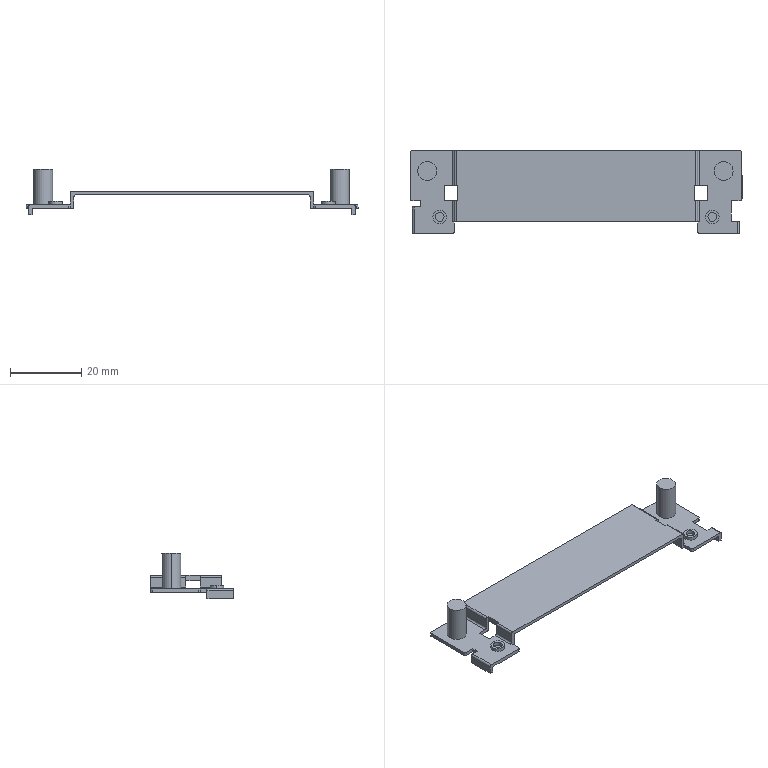Part | SolidWorks | features ICE 7, Attribute 3, Extrusion 1, Fillet 1 | 1 solid | 84 faces | box 93.1 x 23.2 x 12.8 mm | volume 2476 mm3 | plane 48 | cylinder 36 | commonest cylinder face diameters 1 x24 2.5 x4 3.8 x4 5.3 x4